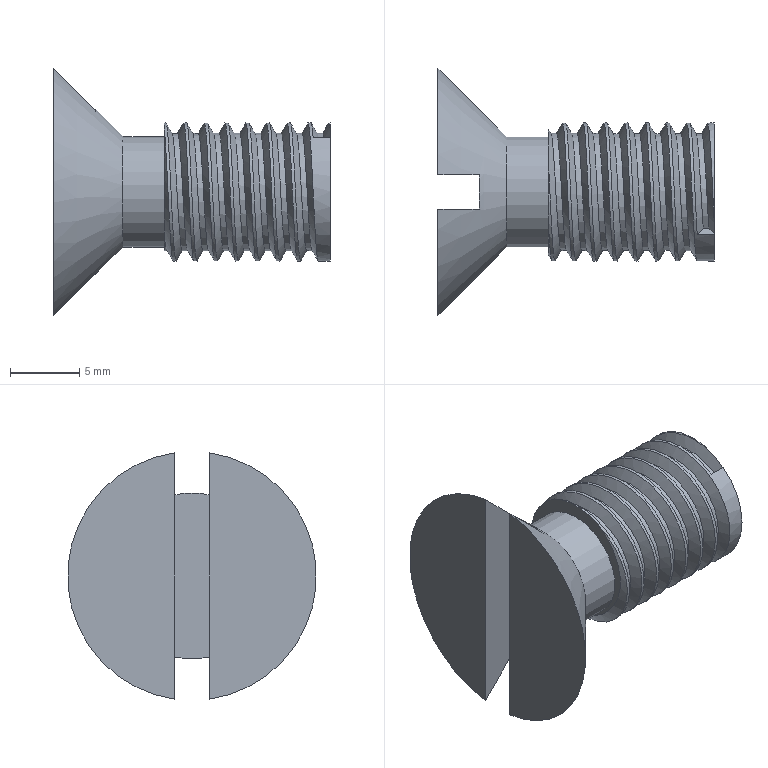Part | NX | features DATUM_CSYS 3, SKETCH 2, EXTRUDE 1, SWP104 1, THREADS 1 | 1 solid | 14 faces | box 20 x 18 x 17.826 mm | volume 1535 mm3 | plane 8 | cylinder 3 | spline 2 | cone 1 | commonest cylinder face diameters 8 x1 8.5 x1 10 x1